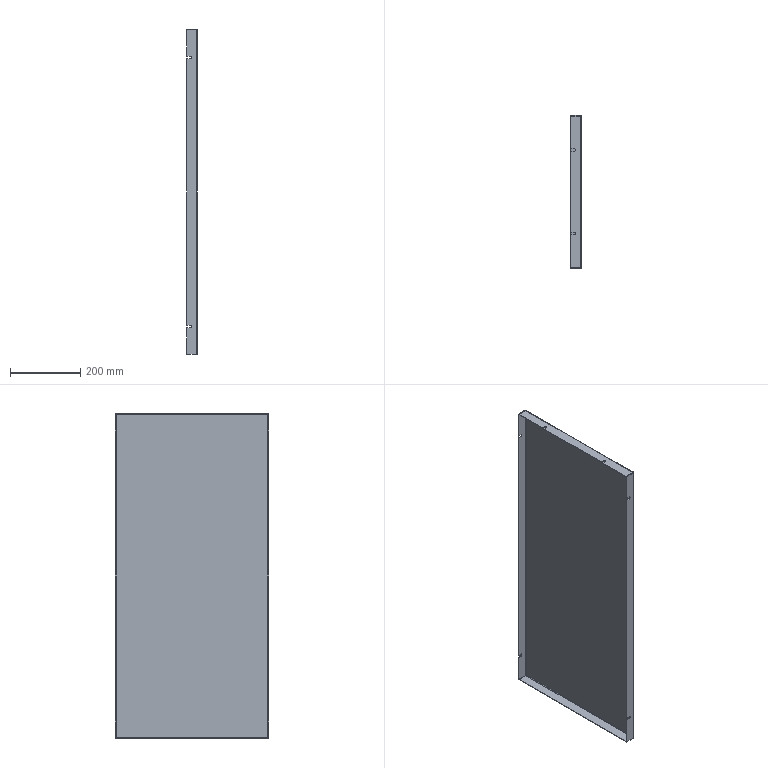Part | STEP file | CSD4-2 | 1 solid | 58 faces | box 30 x 438 x 928 mm | volume 721285 mm3 | plane 44 | cylinder 14 | commonest cylinder face diameters 7 x6 3 x4 6 x4